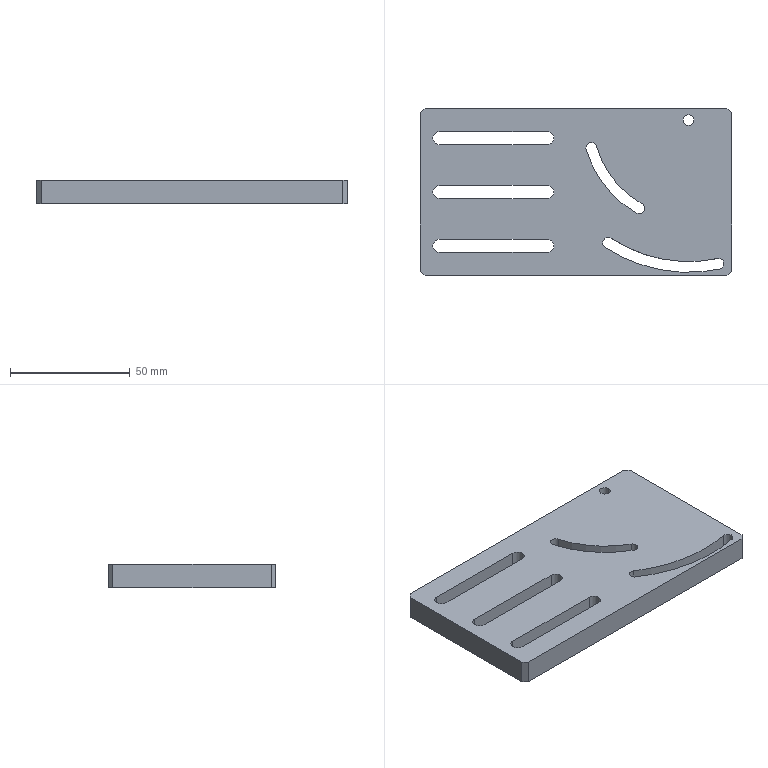Part | NX | 1 solid | 31 faces | box 130 x 70 x 10 mm | volume 78647 mm3 | plane 16 | cylinder 15 | commonest cylinder face diameters 5.5 x6 4.5 x5 79.924 x1 88.924 x1 118.077 x1 127.077 x1
STEP:
#1=CARTESIAN_POINT('',(-63.,35.,10.));
#2=VERTEX_POINT('',#1);
#3=CARTESIAN_POINT('',(-65.,33.,10.));
#4=VERTEX_POINT('',#3);
#5=CARTESIAN_POINT('',(-65.,33.,10.));
#6=DIRECTION('',(-0.7071,-0.7071,0.));
#7=VECTOR('',#6,1000.);
#8=LINE('',#5,#7);
#9=EDGE_CURVE('',#2,#4,#8,.T.);
#10=ORIENTED_EDGE('',*,*,#9,.F.);
#11=CARTESIAN_POINT('',(-63.,35.,0.));
#12=VERTEX_POINT('',#11);
#13=CARTESIAN_POINT('',(-63.,35.,10.));
#14=DIRECTION('',(0.,0.,1.));
#15=VECTOR('',#14,1000.);
#16=LINE('',#13,#15);
#17=EDGE_CURVE('',#12,#2,#16,.T.);
#18=ORIENTED_EDGE('',*,*,#17,.F.);
#19=CARTESIAN_POINT('',(-65.,33.,0.));
#20=VERTEX_POINT('',#19);
#21=CARTESIAN_POINT('',(-49.,49.,0.));
#22=DIRECTION('',(0.7071,0.7071,0.));
#23=VECTOR('',#22,1000.);
#24=LINE('',#21,#23);
#25=EDGE_CURVE('',#20,#12,#24,.T.);
#26=ORIENTED_EDGE('',*,*,#25,.F.);
#27=CARTESIAN_POINT('',(-65.,33.,10.));
#28=DIRECTION('',(0.,0.,-1.));
#29=VECTOR('',#28,1000.);
#30=LINE('',#27,#29);
#31=EDGE_CURVE('',#4,#20,#30,.T.);
#32=ORIENTED_EDGE('',*,*,#31,.F.);
#33=EDGE_LOOP('',(#10,#18,#26,#32));
#34=FACE_BOUND('',#33,.T.);
#35=CARTESIAN_POINT('',(-65.,33.,10.));
#36=DIRECTION('',(0.7071,-0.7071,0.));
#37=DIRECTION('',(0.,0.,-1.));
#38=AXIS2_PLACEMENT_3D('',#35,#36,#37);
#39=PLANE('',#38);
#40=ADVANCED_FACE('',(#34),#39,.F.);
#41=CARTESIAN_POINT('',(-65.,-33.,10.));
#42=VERTEX_POINT('',#41);
#43=CARTESIAN_POINT('',(-63.,-35.,10.));
#44=VERTEX_POINT('',#43);
#45=CARTESIAN_POINT('',(-63.,-35.,10.));
#46=DIRECTION('',(0.7071,-0.7071,0.));
#47=VECTOR('',#46,1000.);
#48=LINE('',#45,#47);
#49=EDGE_CURVE('',#42,#44,#48,.T.);
#50=ORIENTED_EDGE('',*,*,#49,.F.);
#51=CARTESIAN_POINT('',(-65.,-33.,0.));
#52=VERTEX_POINT('',#51);
#53=CARTESIAN_POINT('',(-65.,-33.,10.));
#54=DIRECTION('',(0.,0.,1.));
#55=VECTOR('',#54,1000.);
#56=LINE('',#53,#55);
#57=EDGE_CURVE('',#52,#42,#56,.T.);
#58=ORIENTED_EDGE('',*,*,#57,.F.);
#59=CARTESIAN_POINT('',(-63.,-35.,0.));
#60=VERTEX_POINT('',#59);
#61=CARTESIAN_POINT('',(-49.,-49.,0.));
#62=DIRECTION('',(-0.7071,0.7071,0.));
#63=VECTOR('',#62,1000.);
#64=LINE('',#61,#63);
#65=EDGE_CURVE('',#60,#52,#64,.T.);
#66=ORIENTED_EDGE('',*,*,#65,.F.);
#67=CARTESIAN_POINT('',(-63.,-35.,10.));
#68=DIRECTION('',(0.,0.,-1.));
#69=VECTOR('',#68,1000.);
#70=LINE('',#67,#69);
#71=EDGE_CURVE('',#44,#60,#70,.T.);
#72=ORIENTED_EDGE('',*,*,#71,.F.);
#73=EDGE_LOOP('',(#50,#58,#66,#72));
#74=FACE_BOUND('',#73,.T.);
#75=CARTESIAN_POINT('',(-63.,-35.,10.));
#76=DIRECTION('',(0.7071,0.7071,0.));
#77=DIRECTION('',(0.,0.,-1.));
#78=AXIS2_PLACEMENT_3D('',#75,#76,#77);
#79=PLANE('',#78);
#80=ADVANCED_FACE('',(#74),#79,.F.);
#81=CARTESIAN_POINT('',(65.,33.,10.));
#82=VERTEX_POINT('',#81);
#83=CARTESIAN_POINT('',(63.,35.,10.));
#84=VERTEX_POINT('',#83);
#85=CARTESIAN_POINT('',(63.,35.,10.));
#86=DIRECTION('',(-0.7071,0.7071,0.));
#87=VECTOR('',#86,1000.);
#88=LINE('',#85,#87);
#89=EDGE_CURVE('',#82,#84,#88,.T.);
#90=ORIENTED_EDGE('',*,*,#89,.F.);
#91=CARTESIAN_POINT('',(65.,33.,0.));
#92=VERTEX_POINT('',#91);
#93=CARTESIAN_POINT('',(65.,33.,10.));
#94=DIRECTION('',(0.,0.,1.));
#95=VECTOR('',#94,1000.);
#96=LINE('',#93,#95);
#97=EDGE_CURVE('',#92,#82,#96,.T.);
#98=ORIENTED_EDGE('',*,*,#97,.F.);
#99=CARTESIAN_POINT('',(63.,35.,0.));
#100=VERTEX_POINT('',#99);
#101=CARTESIAN_POINT('',(49.,49.,0.));
#102=DIRECTION('',(0.7071,-0.7071,0.));
#103=VECTOR('',#102,1000.);
#104=LINE('',#101,#103);
#105=EDGE_CURVE('',#100,#92,#104,.T.);
#106=ORIENTED_EDGE('',*,*,#105,.F.);
#107=CARTESIAN_POINT('',(63.,35.,10.));
#108=DIRECTION('',(0.,0.,-1.));
#109=VECTOR('',#108,1000.);
#110=LINE('',#107,#109);
#111=EDGE_CURVE('',#84,#100,#110,.T.);
#112=ORIENTED_EDGE('',*,*,#111,.F.);
#113=EDGE_LOOP('',(#90,#98,#106,#112));
#114=FACE_BOUND('',#113,.T.);
#115=CARTESIAN_POINT('',(63.,35.,10.));
#116=DIRECTION('',(-0.7071,-0.7071,0.));
#117=DIRECTION('',(0.,0.,-1.));
#118=AXIS2_PLACEMENT_3D('',#115,#116,#117);
#119=PLANE('',#118);
#120=ADVANCED_FACE('',(#114),#119,.F.);
#121=CARTESIAN_POINT('',(63.,-35.,10.));
#122=VERTEX_POINT('',#121);
#123=CARTESIAN_POINT('',(65.,-33.,10.));
#124=VERTEX_POINT('',#123);
#125=CARTESIAN_POINT('',(65.,-33.,10.));
#126=DIRECTION('',(0.7071,0.7071,0.));
#127=VECTOR('',#126,1000.);
#128=LINE('',#125,#127);
#129=EDGE_CURVE('',#122,#124,#128,.T.);
#130=ORIENTED_EDGE('',*,*,#129,.F.);
#131=CARTESIAN_POINT('',(63.,-35.,0.));
#132=VERTEX_POINT('',#131);
#133=CARTESIAN_POINT('',(63.,-35.,10.));
#134=DIRECTION('',(0.,0.,1.));
#135=VECTOR('',#134,1000.);
#136=LINE('',#133,#135);
#137=EDGE_CURVE('',#132,#122,#136,.T.);
#138=ORIENTED_EDGE('',*,*,#137,.F.);
#139=CARTESIAN_POINT('',(65.,-33.,0.));
#140=VERTEX_POINT('',#139);
#141=CARTESIAN_POINT('',(49.,-49.,0.));
#142=DIRECTION('',(-0.7071,-0.7071,0.));
#143=VECTOR('',#142,1000.);
#144=LINE('',#141,#143);
#145=EDGE_CURVE('',#140,#132,#144,.T.);
#146=ORIENTED_EDGE('',*,*,#145,.F.);
#147=CARTESIAN_POINT('',(65.,-33.,10.));
#148=DIRECTION('',(0.,0.,-1.));
#149=VECTOR('',#148,1000.);
#150=LINE('',#147,#149);
#151=EDGE_CURVE('',#124,#140,#150,.T.);
#152=ORIENTED_EDGE('',*,*,#151,.F.);
#153=EDGE_LOOP('',(#130,#138,#146,#152));
#154=FACE_BOUND('',#153,.T.);
#155=CARTESIAN_POINT('',(65.,-33.,10.));
#156=DIRECTION('',(-0.7071,0.7071,0.));
#157=DIRECTION('',(0.,0.,-1.));
#158=AXIS2_PLACEMENT_3D('',#155,#156,#157);
#159=PLANE('',#158);
#160=ADVANCED_FACE('',(#154),#159,.F.);
#161=CARTESIAN_POINT('',(-12.,19.75,0.));
#162=VERTEX_POINT('',#161);
#163=CARTESIAN_POINT('',(-57.,19.75,0.));
#164=VERTEX_POINT('',#163);
#165=CARTESIAN_POINT('',(0.,19.75,0.));
#166=DIRECTION('',(-1.,0.,0.));
#167=VECTOR('',#166,1000.);
#168=LINE('',#165,#167);
#169=EDGE_CURVE('',#162,#164,#168,.T.);
#170=ORIENTED_EDGE('',*,*,#169,.T.);
#171=CARTESIAN_POINT('',(-57.,19.75,10.));
#172=VERTEX_POINT('',#171);
#173=CARTESIAN_POINT('',(-57.,19.75,-20.));
#174=DIRECTION('',(0.,0.,1.));
#175=VECTOR('',#174,1000.);
#176=LINE('',#173,#175);
#177=EDGE_CURVE('',#164,#172,#176,.T.);
#178=ORIENTED_EDGE('',*,*,#177,.T.);
#179=CARTESIAN_POINT('',(-12.,19.75,10.));
#180=VERTEX_POINT('',#179);
#181=CARTESIAN_POINT('',(-57.,19.75,10.));
#182=DIRECTION('',(1.,0.,0.));
#183=VECTOR('',#182,1000.);
#184=LINE('',#181,#183);
#185=EDGE_CURVE('',#172,#180,#184,.T.);
#186=ORIENTED_EDGE('',*,*,#185,.T.);
#187=CARTESIAN_POINT('',(-12.,19.75,-20.));
#188=DIRECTION('',(0.,0.,1.));
#189=VECTOR('',#188,1000.);
#190=LINE('',#187,#189);
#191=EDGE_CURVE('',#162,#180,#190,.T.);
#192=ORIENTED_EDGE('',*,*,#191,.F.);
#193=EDGE_LOOP('',(#170,#178,#186,#192));
#194=FACE_BOUND('',#193,.T.);
#195=CARTESIAN_POINT('',(-57.,19.75,-20.));
#196=DIRECTION('',(0.,-1.,0.));
#197=DIRECTION('',(0.,0.,-1.));
#198=AXIS2_PLACEMENT_3D('',#195,#196,#197);
#199=PLANE('',#198);
#200=ADVANCED_FACE('',(#194),#199,.F.);
#201=CARTESIAN_POINT('',(-57.,25.25,0.));
#202=VERTEX_POINT('',#201);
#203=CARTESIAN_POINT('',(-12.,25.25,0.));
#204=VERTEX_POINT('',#203);
#205=CARTESIAN_POINT('',(0.,25.25,0.));
#206=DIRECTION('',(1.,0.,0.));
#207=VECTOR('',#206,1000.);
#208=LINE('',#205,#207);
#209=EDGE_CURVE('',#202,#204,#208,.T.);
#210=ORIENTED_EDGE('',*,*,#209,.T.);
#211=CARTESIAN_POINT('',(-12.,25.25,10.));
#212=VERTEX_POINT('',#211);
#213=CARTESIAN_POINT('',(-12.,25.25,-20.));
#214=DIRECTION('',(0.,0.,1.));
#215=VECTOR('',#214,1000.);
#216=LINE('',#213,#215);
#217=EDGE_CURVE('',#204,#212,#216,.T.);
#218=ORIENTED_EDGE('',*,*,#217,.T.);
#219=CARTESIAN_POINT('',(-57.,25.25,10.));
#220=VERTEX_POINT('',#219);
#221=CARTESIAN_POINT('',(-57.,25.25,10.));
#222=DIRECTION('',(-1.,0.,0.));
#223=VECTOR('',#222,1000.);
#224=LINE('',#221,#223);
#225=EDGE_CURVE('',#212,#220,#224,.T.);
#226=ORIENTED_EDGE('',*,*,#225,.T.);
#227=CARTESIAN_POINT('',(-57.,25.25,-20.));
#228=DIRECTION('',(0.,0.,1.));
#229=VECTOR('',#228,1000.);
#230=LINE('',#227,#229);
#231=EDGE_CURVE('',#202,#220,#230,.T.);
#232=ORIENTED_EDGE('',*,*,#231,.F.);
#233=EDGE_LOOP('',(#210,#218,#226,#232));
#234=FACE_BOUND('',#233,.T.);
#235=CARTESIAN_POINT('',(-57.,25.25,-20.));
#236=DIRECTION('',(0.,1.,0.));
#237=DIRECTION('',(0.,0.,1.));
#238=AXIS2_PLACEMENT_3D('',#235,#236,#237);
#239=PLANE('',#238);
#240=ADVANCED_FACE('',(#234),#239,.F.);
#241=CARTESIAN_POINT('',(-57.,22.5,0.));
#242=DIRECTION('',(0.,0.,-1.));
#243=DIRECTION('',(-1.,0.,0.));
#244=AXIS2_PLACEMENT_3D('',#241,#242,#243);
#245=CIRCLE('',#244,2.75);
#246=EDGE_CURVE('',#164,#202,#245,.T.);
#247=ORIENTED_EDGE('',*,*,#246,.T.);
#248=ORIENTED_EDGE('',*,*,#231,.T.);
#249=CARTESIAN_POINT('',(-57.,22.5,10.));
#250=DIRECTION('',(0.,0.,1.));
#251=DIRECTION('',(1.,0.,0.));
#252=AXIS2_PLACEMENT_3D('',#249,#250,#251);
#253=CIRCLE('',#252,2.75);
#254=EDGE_CURVE('',#220,#172,#253,.T.);
#255=ORIENTED_EDGE('',*,*,#254,.T.);
#256=ORIENTED_EDGE('',*,*,#177,.F.);
#257=EDGE_LOOP('',(#247,#248,#255,#256));
#258=FACE_BOUND('',#257,.T.);
#259=CARTESIAN_POINT('',(-57.,22.5,-20.));
#260=DIRECTION('',(0.,0.,1.));
#261=DIRECTION('',(1.,0.,0.));
#262=AXIS2_PLACEMENT_3D('',#259,#260,#261);
#263=CYLINDRICAL_SURFACE('',#262,2.75);
#264=ADVANCED_FACE('',(#258),#263,.F.);
#265=CARTESIAN_POINT('',(-12.,-25.25,0.));
#266=VERTEX_POINT('',#265);
#267=CARTESIAN_POINT('',(-57.,-25.25,0.));
#268=VERTEX_POINT('',#267);
#269=CARTESIAN_POINT('',(0.,-25.25,0.));
#270=DIRECTION('',(-1.,0.,0.));
#271=VECTOR('',#270,1000.);
#272=LINE('',#269,#271);
#273=EDGE_CURVE('',#266,#268,#272,.T.);
#274=ORIENTED_EDGE('',*,*,#273,.T.);
#275=CARTESIAN_POINT('',(-57.,-25.25,10.));
#276=VERTEX_POINT('',#275);
#277=CARTESIAN_POINT('',(-57.,-25.25,-20.));
#278=DIRECTION('',(0.,0.,1.));
#279=VECTOR('',#278,1000.);
#280=LINE('',#277,#279);
#281=EDGE_CURVE('',#268,#276,#280,.T.);
#282=ORIENTED_EDGE('',*,*,#281,.T.);
#283=CARTESIAN_POINT('',(-12.,-25.25,10.));
#284=VERTEX_POINT('',#283);
#285=CARTESIAN_POINT('',(-57.,-25.25,10.));
#286=DIRECTION('',(1.,0.,0.));
#287=VECTOR('',#286,1000.);
#288=LINE('',#285,#287);
#289=EDGE_CURVE('',#276,#284,#288,.T.);
#290=ORIENTED_EDGE('',*,*,#289,.T.);
#291=CARTESIAN_POINT('',(-12.,-25.25,-20.));
#292=DIRECTION('',(0.,0.,1.));
#293=VECTOR('',#292,1000.);
#294=LINE('',#291,#293);
#295=EDGE_CURVE('',#266,#284,#294,.T.);
#296=ORIENTED_EDGE('',*,*,#295,.F.);
#297=EDGE_LOOP('',(#274,#282,#290,#296));
#298=FACE_BOUND('',#297,.T.);
#299=CARTESIAN_POINT('',(-57.,-25.25,-20.));
#300=DIRECTION('',(0.,-1.,0.));
#301=DIRECTION('',(0.,0.,-1.));
#302=AXIS2_PLACEMENT_3D('',#299,#300,#301);
#303=PLANE('',#302);
#304=ADVANCED_FACE('',(#298),#303,.F.);
#305=CARTESIAN_POINT('',(-57.,-19.75,0.));
#306=VERTEX_POINT('',#305);
#307=CARTESIAN_POINT('',(-12.,-19.75,0.));
#308=VERTEX_POINT('',#307);
#309=CARTESIAN_POINT('',(0.,-19.75,0.));
#310=DIRECTION('',(1.,0.,0.));
#311=VECTOR('',#310,1000.);
#312=LINE('',#309,#311);
#313=EDGE_CURVE('',#306,#308,#312,.T.);
#314=ORIENTED_EDGE('',*,*,#313,.T.);
#315=CARTESIAN_POINT('',(-12.,-19.75,10.));
#316=VERTEX_POINT('',#315);
#317=CARTESIAN_POINT('',(-12.,-19.75,-20.));
#318=DIRECTION('',(0.,0.,1.));
#319=VECTOR('',#318,1000.);
#320=LINE('',#317,#319);
#321=EDGE_CURVE('',#308,#316,#320,.T.);
#322=ORIENTED_EDGE('',*,*,#321,.T.);
#323=CARTESIAN_POINT('',(-57.,-19.75,10.));
#324=VERTEX_POINT('',#323);
#325=CARTESIAN_POINT('',(-57.,-19.75,10.));
#326=DIRECTION('',(-1.,0.,0.));
#327=VECTOR('',#326,1000.);
#328=LINE('',#325,#327);
#329=EDGE_CURVE('',#316,#324,#328,.T.);
#330=ORIENTED_EDGE('',*,*,#329,.T.);
#331=CARTESIAN_POINT('',(-57.,-19.75,-20.));
#332=DIRECTION('',(0.,0.,1.));
#333=VECTOR('',#332,1000.);
#334=LINE('',#331,#333);
#335=EDGE_CURVE('',#306,#324,#334,.T.);
#336=ORIENTED_EDGE('',*,*,#335,.F.);
#337=EDGE_LOOP('',(#314,#322,#330,#336));
#338=FACE_BOUND('',#337,.T.);
#339=CARTESIAN_POINT('',(-57.,-19.75,-20.));
#340=DIRECTION('',(0.,1.,0.));
#341=DIRECTION('',(0.,0.,1.));
#342=AXIS2_PLACEMENT_3D('',#339,#340,#341);
#343=PLANE('',#342);
#344=ADVANCED_FACE('',(#338),#343,.F.);
#345=CARTESIAN_POINT('',(-57.,-22.5,0.));
#346=DIRECTION('',(0.,0.,-1.));
#347=DIRECTION('',(-1.,0.,0.));
#348=AXIS2_PLACEMENT_3D('',#345,#346,#347);
#349=CIRCLE('',#348,2.75);
#350=EDGE_CURVE('',#268,#306,#349,.T.);
#351=ORIENTED_EDGE('',*,*,#350,.T.);
#352=ORIENTED_EDGE('',*,*,#335,.T.);
#353=CARTESIAN_POINT('',(-57.,-22.5,10.));
#354=DIRECTION('',(0.,0.,1.));
#355=DIRECTION('',(-1.,0.,0.));
#356=AXIS2_PLACEMENT_3D('',#353,#354,#355);
#357=CIRCLE('',#356,2.75);
#358=EDGE_CURVE('',#324,#276,#357,.T.);
#359=ORIENTED_EDGE('',*,*,#358,.T.);
#360=ORIENTED_EDGE('',*,*,#281,.F.);
#361=EDGE_LOOP('',(#351,#352,#359,#360));
#362=FACE_BOUND('',#361,.T.);
#363=CARTESIAN_POINT('',(-57.,-22.5,-20.));
#364=DIRECTION('',(0.,0.,1.));
#365=DIRECTION('',(1.,0.,0.));
#366=AXIS2_PLACEMENT_3D('',#363,#364,#365);
#367=CYLINDRICAL_SURFACE('',#366,2.75);
#368=ADVANCED_FACE('',(#362),#367,.F.);
#369=CARTESIAN_POINT('',(-12.,-2.75,0.));
#370=VERTEX_POINT('',#369);
#371=CARTESIAN_POINT('',(-57.,-2.75,0.));
#372=VERTEX_POINT('',#371);
#373=CARTESIAN_POINT('',(0.,-2.75,0.));
#374=DIRECTION('',(-1.,0.,0.));
#375=VECTOR('',#374,1000.);
#376=LINE('',#373,#375);
#377=EDGE_CURVE('',#370,#372,#376,.T.);
#378=ORIENTED_EDGE('',*,*,#377,.T.);
#379=CARTESIAN_POINT('',(-57.,-2.75,10.));
#380=VERTEX_POINT('',#379);
#381=CARTESIAN_POINT('',(-57.,-2.75,-20.));
#382=DIRECTION('',(0.,0.,1.));
#383=VECTOR('',#382,1000.);
#384=LINE('',#381,#383);
#385=EDGE_CURVE('',#372,#380,#384,.T.);
#386=ORIENTED_EDGE('',*,*,#385,.T.);
#387=CARTESIAN_POINT('',(-12.,-2.75,10.));
#388=VERTEX_POINT('',#387);
#389=CARTESIAN_POINT('',(-57.,-2.75,10.));
#390=DIRECTION('',(1.,0.,0.));
#391=VECTOR('',#390,1000.);
#392=LINE('',#389,#391);
#393=EDGE_CURVE('',#380,#388,#392,.T.);
#394=ORIENTED_EDGE('',*,*,#393,.T.);
#395=CARTESIAN_POINT('',(-12.,-2.75,-20.));
#396=DIRECTION('',(0.,0.,1.));
#397=VECTOR('',#396,1000.);
#398=LINE('',#395,#397);
#399=EDGE_CURVE('',#370,#388,#398,.T.);
#400=ORIENTED_EDGE('',*,*,#399,.F.);
#401=EDGE_LOOP('',(#378,#386,#394,#400));
#402=FACE_BOUND('',#401,.T.);
#403=CARTESIAN_POINT('',(-57.,-2.75,-20.));
#404=DIRECTION('',(0.,-1.,0.));
#405=DIRECTION('',(0.,0.,-1.));
#406=AXIS2_PLACEMENT_3D('',#403,#404,#405);
#407=PLANE('',#406);
#408=ADVANCED_FACE('',(#402),#407,.F.);
#409=CARTESIAN_POINT('',(-57.,2.75,0.));
#410=VERTEX_POINT('',#409);
#411=CARTESIAN_POINT('',(-12.,2.75,0.));
#412=VERTEX_POINT('',#411);
#413=CARTESIAN_POINT('',(0.,2.75,0.));
#414=DIRECTION('',(1.,0.,0.));
#415=VECTOR('',#414,1000.);
#416=LINE('',#413,#415);
#417=EDGE_CURVE('',#410,#412,#416,.T.);
#418=ORIENTED_EDGE('',*,*,#417,.T.);
#419=CARTESIAN_POINT('',(-12.,2.75,10.));
#420=VERTEX_POINT('',#419);
#421=CARTESIAN_POINT('',(-12.,2.75,-20.));
#422=DIRECTION('',(0.,0.,1.));
#423=VECTOR('',#422,1000.);
#424=LINE('',#421,#423);
#425=EDGE_CURVE('',#412,#420,#424,.T.);
#426=ORIENTED_EDGE('',*,*,#425,.T.);
#427=CARTESIAN_POINT('',(-57.,2.75,10.));
#428=VERTEX_POINT('',#427);
#429=CARTESIAN_POINT('',(-57.,2.75,10.));
#430=DIRECTION('',(-1.,0.,0.));
#431=VECTOR('',#430,1000.);
#432=LINE('',#429,#431);
#433=EDGE_CURVE('',#420,#428,#432,.T.);
#434=ORIENTED_EDGE('',*,*,#433,.T.);
#435=CARTESIAN_POINT('',(-57.,2.75,-20.));
#436=DIRECTION('',(0.,0.,1.));
#437=VECTOR('',#436,1000.);
#438=LINE('',#435,#437);
#439=EDGE_CURVE('',#410,#428,#438,.T.);
#440=ORIENTED_EDGE('',*,*,#439,.F.);
#441=EDGE_LOOP('',(#418,#426,#434,#440));
#442=FACE_BOUND('',#441,.T.);
#443=CARTESIAN_POINT('',(-57.,2.75,-20.));
#444=DIRECTION('',(0.,1.,0.));
#445=DIRECTION('',(0.,0.,1.));
#446=AXIS2_PLACEMENT_3D('',#443,#444,#445);
#447=PLANE('',#446);
#448=ADVANCED_FACE('',(#442),#447,.F.);
#449=CARTESIAN_POINT('',(-57.,0.,0.));
#450=DIRECTION('',(0.,0.,-1.));
#451=DIRECTION('',(-1.,0.,0.));
#452=AXIS2_PLACEMENT_3D('',#449,#450,#451);
#453=CIRCLE('',#452,2.75);
#454=EDGE_CURVE('',#372,#410,#453,.T.);
#455=ORIENTED_EDGE('',*,*,#454,.T.);
#456=ORIENTED_EDGE('',*,*,#439,.T.);
#457=CARTESIAN_POINT('',(-57.,0.,10.));
#458=DIRECTION('',(0.,0.,1.));
#459=DIRECTION('',(1.,0.,0.));
#460=AXIS2_PLACEMENT_3D('',#457,#458,#459);
#461=CIRCLE('',#460,2.75);
#462=EDGE_CURVE('',#428,#380,#461,.T.);
#463=ORIENTED_EDGE('',*,*,#462,.T.);
#464=ORIENTED_EDGE('',*,*,#385,.F.);
#465=EDGE_LOOP('',(#455,#456,#463,#464));
#466=FACE_BOUND('',#465,.T.);
#467=CARTESIAN_POINT('',(-57.,0.,-20.));
#468=DIRECTION('',(0.,0.,1.));
#469=DIRECTION('',(1.,0.,0.));
#470=AXIS2_PLACEMENT_3D('',#467,#468,#469);
#471=CYLINDRICAL_SURFACE('',#470,2.75);
#472=ADVANCED_FACE('',(#466),#471,.F.);
#473=CARTESIAN_POINT('',(14.645,-19.383,0.));
#474=VERTEX_POINT('',#473);
#475=CARTESIAN_POINT('',(59.041,-27.797,0.));
#476=VERTEX_POINT('',#475);
#477=CARTESIAN_POINT('',(47.,30.,0.));
#478=DIRECTION('',(0.,0.,1.));
#479=DIRECTION('',(-1.,0.,0.));
#480=AXIS2_PLACEMENT_3D('',#477,#478,#479);
#481=CIRCLE('',#480,59.038);
#482=EDGE_CURVE('',#474,#476,#481,.T.);
#483=ORIENTED_EDGE('',*,*,#482,.T.);
#484=CARTESIAN_POINT('',(59.041,-27.797,10.));
#485=VERTEX_POINT('',#484);
#486=CARTESIAN_POINT('',(59.041,-27.797,5.));
#487=DIRECTION('',(0.,0.,1.));
#488=VECTOR('',#487,1000.);
#489=LINE('',#486,#488);
#490=EDGE_CURVE('',#476,#485,#489,.T.);
#491=ORIENTED_EDGE('',*,*,#490,.T.);
#492=CARTESIAN_POINT('',(14.645,-19.383,10.));
#493=VERTEX_POINT('',#492);
#494=CARTESIAN_POINT('',(47.,30.,10.));
#495=DIRECTION('',(0.,0.,-1.));
#496=DIRECTION('',(1.,0.,0.));
#497=AXIS2_PLACEMENT_3D('',#494,#495,#496);
#498=CIRCLE('',#497,59.038);
#499=EDGE_CURVE('',#485,#493,#498,.T.);
#500=ORIENTED_EDGE('',*,*,#499,.T.);
#501=CARTESIAN_POINT('',(14.645,-19.383,-20.));
#502=DIRECTION('',(0.,0.,1.));
#503=VECTOR('',#502,1000.);
#504=LINE('',#501,#503);
#505=EDGE_CURVE('',#474,#493,#504,.T.);
#506=ORIENTED_EDGE('',*,*,#505,.F.);
#507=EDGE_LOOP('',(#483,#491,#500,#506));
#508=FACE_BOUND('',#507,.T.);
#509=CARTESIAN_POINT('',(47.,30.,-20.));
#510=DIRECTION('',(0.,0.,1.));
#511=DIRECTION('',(1.,0.,0.));
#512=AXIS2_PLACEMENT_3D('',#509,#510,#511);
#513=CYLINDRICAL_SURFACE('',#512,59.038);
#514=ADVANCED_FACE('',(#508),#513,.T.);
#515=CARTESIAN_POINT('',(12.179,-23.147,0.));
#516=VERTEX_POINT('',#515);
#517=CARTESIAN_POINT('',(13.412,-21.265,0.));
#518=DIRECTION('',(0.,0.,-1.));
#519=DIRECTION('',(-1.,0.,0.));
#520=AXIS2_PLACEMENT_3D('',#517,#518,#519);
#521=CIRCLE('',#520,2.25);
#522=EDGE_CURVE('',#516,#474,#521,.T.);
#523=ORIENTED_EDGE('',*,*,#522,.T.);
#524=ORIENTED_EDGE('',*,*,#505,.T.);
#525=CARTESIAN_POINT('',(12.179,-23.147,10.));
#526=VERTEX_POINT('',#525);
#527=CARTESIAN_POINT('',(13.412,-21.265,10.));
#528=DIRECTION('',(0.,0.,1.));
#529=DIRECTION('',(1.,0.,0.));
#530=AXIS2_PLACEMENT_3D('',#527,#528,#529);
#531=CIRCLE('',#530,2.25);
#532=EDGE_CURVE('',#493,#526,#531,.T.);
#533=ORIENTED_EDGE('',*,*,#532,.T.);
#534=CARTESIAN_POINT('',(12.179,-23.147,-20.));
#535=DIRECTION('',(0.,0.,1.));
#536=VECTOR('',#535,1000.);
#537=LINE('',#534,#536);
#538=EDGE_CURVE('',#516,#526,#537,.T.);
#539=ORIENTED_EDGE('',*,*,#538,.F.);
#540=EDGE_LOOP('',(#523,#524,#533,#539));
#541=FACE_BOUND('',#540,.T.);
#542=CARTESIAN_POINT('',(13.412,-21.265,-20.));
#543=DIRECTION('',(0.,0.,1.));
#544=DIRECTION('',(1.,0.,0.));
#545=AXIS2_PLACEMENT_3D('',#542,#543,#544);
#546=CYLINDRICAL_SURFACE('',#545,2.25);
#547=ADVANCED_FACE('',(#541),#546,.F.);
#548=CARTESIAN_POINT('',(59.959,-32.203,0.));
#549=VERTEX_POINT('',#548);
#550=CARTESIAN_POINT('',(47.,30.,0.));
#551=DIRECTION('',(0.,0.,-1.));
#552=DIRECTION('',(-1.,0.,0.));
#553=AXIS2_PLACEMENT_3D('',#550,#551,#552);
#554=CIRCLE('',#553,63.538);
#555=EDGE_CURVE('',#549,#516,#554,.T.);
#556=ORIENTED_EDGE('',*,*,#555,.T.);
#557=ORIENTED_EDGE('',*,*,#538,.T.);
#558=CARTESIAN_POINT('',(59.959,-32.203,10.));
#559=VERTEX_POINT('',#558);
#560=CARTESIAN_POINT('',(47.,30.,10.));
#561=DIRECTION('',(0.,0.,1.));
#562=DIRECTION('',(1.,0.,0.));
#563=AXIS2_PLACEMENT_3D('',#560,#561,#562);
#564=CIRCLE('',#563,63.538);
#565=EDGE_CURVE('',#526,#559,#564,.T.);
#566=ORIENTED_EDGE('',*,*,#565,.T.);
#567=CARTESIAN_POINT('',(59.959,-32.203,-5.));
#568=DIRECTION('',(0.,0.,1.));
#569=VECTOR('',#568,1000.);
#570=LINE('',#567,#569);
#571=EDGE_CURVE('',#549,#559,#570,.T.);
#572=ORIENTED_EDGE('',*,*,#571,.F.);
#573=EDGE_LOOP('',(#556,#557,#566,#572));
#574=FACE_BOUND('',#573,.T.);
#575=CARTESIAN_POINT('',(47.,30.,-20.));
#576=DIRECTION('',(0.,0.,1.));
#577=DIRECTION('',(1.,0.,0.));
#578=AXIS2_PLACEMENT_3D('',#575,#576,#577);
#579=CYLINDRICAL_SURFACE('',#578,63.538);
#580=ADVANCED_FACE('',(#574),#579,.F.);
#581=CARTESIAN_POINT('',(8.575,19.022,0.));
#582=VERTEX_POINT('',#581);
#583=CARTESIAN_POINT('',(27.593,-4.933,0.));
#584=VERTEX_POINT('',#583);
#585=CARTESIAN_POINT('',(47.,30.,0.));
#586=DIRECTION('',(0.,0.,1.));
#587=DIRECTION('',(-1.,0.,0.));
#588=AXIS2_PLACEMENT_3D('',#585,#586,#587);
#589=CIRCLE('',#588,39.962);
#590=EDGE_CURVE('',#582,#584,#589,.T.);
#591=ORIENTED_EDGE('',*,*,#590,.T.);
#592=CARTESIAN_POINT('',(27.593,-4.933,10.));
#593=VERTEX_POINT('',#592);
#594=CARTESIAN_POINT('',(27.593,-4.933,5.));
#595=DIRECTION('',(0.,0.,1.));
#596=VECTOR('',#595,1000.);
#597=LINE('',#594,#596);
#598=EDGE_CURVE('',#584,#593,#597,.T.);
#599=ORIENTED_EDGE('',*,*,#598,.T.);
#600=CARTESIAN_POINT('',(8.575,19.022,10.));
#601=VERTEX_POINT('',#600);
#602=CARTESIAN_POINT('',(47.,30.,10.));
#603=DIRECTION('',(0.,0.,-1.));
#604=DIRECTION('',(1.,0.,0.));
#605=AXIS2_PLACEMENT_3D('',#602,#603,#604);
#606=CIRCLE('',#605,39.962);
#607=EDGE_CURVE('',#593,#601,#606,.T.);
#608=ORIENTED_EDGE('',*,*,#607,.T.);
#609=CARTESIAN_POINT('',(8.575,19.022,-20.));
#610=DIRECTION('',(0.,0.,1.));
#611=VECTOR('',#610,1000.);
#612=LINE('',#609,#611);
#613=EDGE_CURVE('',#582,#601,#612,.T.);
#614=ORIENTED_EDGE('',*,*,#613,.F.);
#615=EDGE_LOOP('',(#591,#599,#608,#614));
#616=FACE_BOUND('',#615,.T.);
#617=CARTESIAN_POINT('',(47.,30.,-20.));
#618=DIRECTION('',(0.,0.,1.));
#619=DIRECTION('',(1.,0.,0.));
#620=AXIS2_PLACEMENT_3D('',#617,#618,#619);
#621=CYLINDRICAL_SURFACE('',#620,39.962);
#622=ADVANCED_FACE('',(#616),#621,.T.);
#623=CARTESIAN_POINT('',(4.249,17.785,0.));
#624=VERTEX_POINT('',#623);
#625=CARTESIAN_POINT('',(6.412,18.403,0.));
#626=DIRECTION('',(0.,0.,-1.));
#627=DIRECTION('',(-1.,0.,0.));
#628=AXIS2_PLACEMENT_3D('',#625,#626,#627);
#629=CIRCLE('',#628,2.25);
#630=EDGE_CURVE('',#624,#582,#629,.T.);
#631=ORIENTED_EDGE('',*,*,#630,.T.);
#632=ORIENTED_EDGE('',*,*,#613,.T.);
#633=CARTESIAN_POINT('',(4.249,17.785,10.));
#634=VERTEX_POINT('',#633);
#635=CARTESIAN_POINT('',(6.412,18.403,10.));
#636=DIRECTION('',(0.,0.,1.));
#637=DIRECTION('',(1.,0.,0.));
#638=AXIS2_PLACEMENT_3D('',#635,#636,#637);
#639=CIRCLE('',#638,2.25);
#640=EDGE_CURVE('',#601,#634,#639,.T.);
#641=ORIENTED_EDGE('',*,*,#640,.T.);
#642=CARTESIAN_POINT('',(4.249,17.785,-20.));
#643=DIRECTION('',(0.,0.,1.));
#644=VECTOR('',#643,1000.);
#645=LINE('',#642,#644);
#646=EDGE_CURVE('',#624,#634,#645,.T.);
#647=ORIENTED_EDGE('',*,*,#646,.F.);
#648=EDGE_LOOP('',(#631,#632,#641,#647));
#649=FACE_BOUND('',#648,.T.);
#650=CARTESIAN_POINT('',(6.412,18.403,-20.));
#651=DIRECTION('',(0.,0.,1.));
#652=DIRECTION('',(1.,0.,0.));
#653=AXIS2_PLACEMENT_3D('',#650,#651,#652);
#654=CYLINDRICAL_SURFACE('',#653,2.25);
#655=ADVANCED_FACE('',(#649),#654,.F.);
#656=CARTESIAN_POINT('',(25.407,-8.867,0.));
#657=VERTEX_POINT('',#656);
#658=CARTESIAN_POINT('',(47.,30.,0.));
#659=DIRECTION('',(0.,0.,-1.));
#660=DIRECTION('',(-1.,0.,0.));
#661=AXIS2_PLACEMENT_3D('',#658,#659,#660);
#662=CIRCLE('',#661,44.462);
#663=EDGE_CURVE('',#657,#624,#662,.T.);
#664=ORIENTED_EDGE('',*,*,#663,.T.);
#665=ORIENTED_EDGE('',*,*,#646,.T.);
#666=CARTESIAN_POINT('',(25.407,-8.867,10.));
#667=VERTEX_POINT('',#666);
#668=CARTESIAN_POINT('',(47.,30.,10.));
#669=DIRECTION('',(0.,0.,1.));
#670=DIRECTION('',(1.,0.,0.));
#671=AXIS2_PLACEMENT_3D('',#668,#669,#670);
#672=CIRCLE('',#671,44.462);
#673=EDGE_CURVE('',#634,#667,#672,.T.);
#674=ORIENTED_EDGE('',*,*,#673,.T.);
#675=CARTESIAN_POINT('',(25.407,-8.867,-5.));
#676=DIRECTION('',(0.,0.,1.));
#677=VECTOR('',#676,1000.);
#678=LINE('',#675,#677);
#679=EDGE_CURVE('',#657,#667,#678,.T.);
#680=ORIENTED_EDGE('',*,*,#679,.F.);
#681=EDGE_LOOP('',(#664,#665,#674,#680));
#682=FACE_BOUND('',#681,.T.);
#683=CARTESIAN_POINT('',(47.,30.,-20.));
#684=DIRECTION('',(0.,0.,1.));
#685=DIRECTION('',(1.,0.,0.));
#686=AXIS2_PLACEMENT_3D('',#683,#684,#685);
#687=CYLINDRICAL_SURFACE('',#686,44.462);
#688=ADVANCED_FACE('',(#682),#687,.F.);
#689=CARTESIAN_POINT('',(-65.,-35.,0.));
#690=DIRECTION('',(1.,0.,0.));
#691=VECTOR('',#690,1000.);
#692=LINE('',#689,#691);
#693=EDGE_CURVE('',#60,#132,#692,.T.);
#694=ORIENTED_EDGE('',*,*,#693,.T.);
#695=ORIENTED_EDGE('',*,*,#137,.T.);
#696=CARTESIAN_POINT('',(-65.,-35.,10.));
#697=DIRECTION('',(1.,0.,0.));
#698=VECTOR('',#697,1000.);
#699=LINE('',#696,#698);
#700=EDGE_CURVE('',#44,#122,#699,.T.);
#701=ORIENTED_EDGE('',*,*,#700,.F.);
#702=ORIENTED_EDGE('',*,*,#71,.T.);
#703=EDGE_LOOP('',(#694,#695,#701,#702));
#704=FACE_BOUND('',#703,.T.);
#705=CARTESIAN_POINT('',(-65.,-35.,10.));
#706=DIRECTION('',(0.,1.,0.));
#707=DIRECTION('',(0.,0.,1.));
#708=AXIS2_PLACEMENT_3D('',#705,#706,#707);
#709=PLANE('',#708);
#710=ADVANCED_FACE('',(#704),#709,.F.);
#711=CARTESIAN_POINT('',(-65.,-35.,0.));
#712=DIRECTION('',(0.,-1.,0.));
#713=VECTOR('',#712,1000.);
#714=LINE('',#711,#713);
#715=EDGE_CURVE('',#20,#52,#714,.T.);
#716=ORIENTED_EDGE('',*,*,#715,.T.);
#717=ORIENTED_EDGE('',*,*,#57,.T.);
#718=CARTESIAN_POINT('',(-65.,-35.,10.));
#719=DIRECTION('',(0.,-1.,0.));
#720=VECTOR('',#719,1000.);
#721=LINE('',#718,#720);
#722=EDGE_CURVE('',#4,#42,#721,.T.);
#723=ORIENTED_EDGE('',*,*,#722,.F.);
#724=ORIENTED_EDGE('',*,*,#31,.T.);
#725=EDGE_LOOP('',(#716,#717,#723,#724));
#726=FACE_BOUND('',#725,.T.);
#727=CARTESIAN_POINT('',(-65.,-35.,10.));
#728=DIRECTION('',(1.,0.,0.));
#729=DIRECTION('',(0.,0.,-1.));
#730=AXIS2_PLACEMENT_3D('',#727,#728,#729);
#731=PLANE('',#730);
#732=ADVANCED_FACE('',(#726),#731,.F.);
#733=CARTESIAN_POINT('',(-65.,35.,10.));
#734=DIRECTION('',(-1.,0.,0.));
#735=VECTOR('',#734,1000.);
#736=LINE('',#733,#735);
#737=EDGE_CURVE('',#84,#2,#736,.T.);
#738=ORIENTED_EDGE('',*,*,#737,.F.);
#739=ORIENTED_EDGE('',*,*,#111,.T.);
#740=CARTESIAN_POINT('',(-65.,35.,0.));
#741=DIRECTION('',(-1.,0.,0.));
#742=VECTOR('',#741,1000.);
#743=LINE('',#740,#742);
#744=EDGE_CURVE('',#100,#12,#743,.T.);
#745=ORIENTED_EDGE('',*,*,#744,.T.);
#746=ORIENTED_EDGE('',*,*,#17,.T.);
#747=EDGE_LOOP('',(#738,#739,#745,#746));
#748=FACE_BOUND('',#747,.T.);
#749=CARTESIAN_POINT('',(-65.,35.,10.));
#750=DIRECTION('',(0.,-1.,0.));
#751=DIRECTION('',(0.,0.,-1.));
#752=AXIS2_PLACEMENT_3D('',#749,#750,#751);
#753=PLANE('',#752);
#754=ADVANCED_FACE('',(#748),#753,.F.);
#755=CARTESIAN_POINT('',(65.,-35.,10.));
#756=DIRECTION('',(0.,1.,0.));
#757=VECTOR('',#756,1000.);
#758=LINE('',#755,#757);
#759=EDGE_CURVE('',#124,#82,#758,.T.);
#760=ORIENTED_EDGE('',*,*,#759,.F.);
#761=ORIENTED_EDGE('',*,*,#151,.T.);
#762=CARTESIAN_POINT('',(65.,-35.,0.));
#763=DIRECTION('',(0.,1.,0.));
#764=VECTOR('',#763,1000.);
#765=LINE('',#762,#764);
#766=EDGE_CURVE('',#140,#92,#765,.T.);
#767=ORIENTED_EDGE('',*,*,#766,.T.);
#768=ORIENTED_EDGE('',*,*,#97,.T.);
#769=EDGE_LOOP('',(#760,#761,#767,#768));
#770=FACE_BOUND('',#769,.T.);
#771=CARTESIAN_POINT('',(65.,-35.,10.));
#772=DIRECTION('',(-1.,0.,0.));
#773=DIRECTION('',(0.,0.,1.));
#774=AXIS2_PLACEMENT_3D('',#771,#772,#773);
#775=PLANE('',#774);
#776=ADVANCED_FACE('',(#770),#775,.F.);
#777=ORIENTED_EDGE('',*,*,#555,.F.);
#778=CARTESIAN_POINT('',(59.5,-30.,0.));
#779=DIRECTION('',(0.,0.,-1.));
#780=DIRECTION('',(-1.,0.,0.));
#781=AXIS2_PLACEMENT_3D('',#778,#779,#780);
#782=CIRCLE('',#781,2.25);
#783=EDGE_CURVE('',#476,#549,#782,.T.);
#784=ORIENTED_EDGE('',*,*,#783,.F.);
#785=ORIENTED_EDGE('',*,*,#482,.F.);
#786=ORIENTED_EDGE('',*,*,#522,.F.);
#787=EDGE_LOOP('',(#777,#784,#785,#786));
#788=FACE_BOUND('',#787,.T.);
#789=ORIENTED_EDGE('',*,*,#766,.F.);
#790=ORIENTED_EDGE('',*,*,#145,.T.);
#791=ORIENTED_EDGE('',*,*,#693,.F.);
#792=ORIENTED_EDGE('',*,*,#65,.T.);
#793=ORIENTED_EDGE('',*,*,#715,.F.);
#794=ORIENTED_EDGE('',*,*,#25,.T.);
#795=ORIENTED_EDGE('',*,*,#744,.F.);
#796=ORIENTED_EDGE('',*,*,#105,.T.);
#797=EDGE_LOOP('',(#789,#790,#791,#792,#793,#794,#795,#796));
#798=FACE_BOUND('',#797,.T.);
#799=CARTESIAN_POINT('',(44.75,30.,0.));
#800=VERTEX_POINT('',#799);
#801=CARTESIAN_POINT('',(47.,30.,0.));
#802=DIRECTION('',(0.,0.,-1.));
#803=DIRECTION('',(-1.,0.,0.));
#804=AXIS2_PLACEMENT_3D('',#801,#802,#803);
#805=CIRCLE('',#804,2.25);
#806=EDGE_CURVE('',#800,#800,#805,.T.);
#807=ORIENTED_EDGE('',*,*,#806,.F.);
#808=EDGE_LOOP('',(#807));
#809=FACE_BOUND('',#808,.T.);
#810=ORIENTED_EDGE('',*,*,#663,.F.);
#811=CARTESIAN_POINT('',(26.5,-6.9,0.));
#812=DIRECTION('',(0.,0.,-1.));
#813=DIRECTION('',(-1.,0.,0.));
#814=AXIS2_PLACEMENT_3D('',#811,#812,#813);
#815=CIRCLE('',#814,2.25);
#816=EDGE_CURVE('',#584,#657,#815,.T.);
#817=ORIENTED_EDGE('',*,*,#816,.F.);
#818=ORIENTED_EDGE('',*,*,#590,.F.);
#819=ORIENTED_EDGE('',*,*,#630,.F.);
#820=EDGE_LOOP('',(#810,#817,#818,#819));
#821=FACE_BOUND('',#820,.T.);
#822=ORIENTED_EDGE('',*,*,#454,.F.);
#823=ORIENTED_EDGE('',*,*,#377,.F.);
#824=CARTESIAN_POINT('',(-12.,0.,0.));
#825=DIRECTION('',(0.,0.,-1.));
#826=DIRECTION('',(-1.,0.,0.));
#827=AXIS2_PLACEMENT_3D('',#824,#825,#826);
#828=CIRCLE('',#827,2.75);
#829=EDGE_CURVE('',#412,#370,#828,.T.);
#830=ORIENTED_EDGE('',*,*,#829,.F.);
#831=ORIENTED_EDGE('',*,*,#417,.F.);
#832=EDGE_LOOP('',(#822,#823,#830,#831));
#833=FACE_BOUND('',#832,.T.);
#834=ORIENTED_EDGE('',*,*,#350,.F.);
#835=ORIENTED_EDGE('',*,*,#273,.F.);
#836=CARTESIAN_POINT('',(-12.,-22.5,0.));
#837=DIRECTION('',(0.,0.,-1.));
#838=DIRECTION('',(-1.,0.,0.));
#839=AXIS2_PLACEMENT_3D('',#836,#837,#838);
#840=CIRCLE('',#839,2.75);
#841=EDGE_CURVE('',#308,#266,#840,.T.);
#842=ORIENTED_EDGE('',*,*,#841,.F.);
#843=ORIENTED_EDGE('',*,*,#313,.F.);
#844=EDGE_LOOP('',(#834,#835,#842,#843));
#845=FACE_BOUND('',#844,.T.);
#846=ORIENTED_EDGE('',*,*,#246,.F.);
#847=ORIENTED_EDGE('',*,*,#169,.F.);
#848=CARTESIAN_POINT('',(-12.,22.5,0.));
#849=DIRECTION('',(0.,0.,-1.));
#850=DIRECTION('',(-1.,0.,0.));
#851=AXIS2_PLACEMENT_3D('',#848,#849,#850);
#852=CIRCLE('',#851,2.75);
#853=EDGE_CURVE('',#204,#162,#852,.T.);
#854=ORIENTED_EDGE('',*,*,#853,.F.);
#855=ORIENTED_EDGE('',*,*,#209,.F.);
#856=EDGE_LOOP('',(#846,#847,#854,#855));
#857=FACE_BOUND('',#856,.T.);
#858=CARTESIAN_POINT('',(0.,0.,0.));
#859=DIRECTION('',(0.,0.,-1.));
#860=DIRECTION('',(-1.,0.,0.));
#861=AXIS2_PLACEMENT_3D('',#858,#859,#860);
#862=PLANE('',#861);
#863=ADVANCED_FACE('',(#788,#798,#809,#821,#833,#845,#857),#862,.T.);
#864=CARTESIAN_POINT('',(59.5,-30.,10.));
#865=DIRECTION('',(0.,0.,1.));
#866=DIRECTION('',(1.,0.,0.));
#867=AXIS2_PLACEMENT_3D('',#864,#865,#866);
#868=CIRCLE('',#867,2.25);
#869=EDGE_CURVE('',#559,#485,#868,.T.);
#870=ORIENTED_EDGE('',*,*,#869,.F.);
#871=ORIENTED_EDGE('',*,*,#565,.F.);
#872=ORIENTED_EDGE('',*,*,#532,.F.);
#873=ORIENTED_EDGE('',*,*,#499,.F.);
#874=EDGE_LOOP('',(#870,#871,#872,#873));
#875=FACE_BOUND('',#874,.T.);
#876=CARTESIAN_POINT('',(26.5,-6.9,10.));
#877=DIRECTION('',(0.,0.,1.));
#878=DIRECTION('',(1.,0.,0.));
#879=AXIS2_PLACEMENT_3D('',#876,#877,#878);
#880=CIRCLE('',#879,2.25);
#881=EDGE_CURVE('',#667,#593,#880,.T.);
#882=ORIENTED_EDGE('',*,*,#881,.F.);
#883=ORIENTED_EDGE('',*,*,#673,.F.);
#884=ORIENTED_EDGE('',*,*,#640,.F.);
#885=ORIENTED_EDGE('',*,*,#607,.F.);
#886=EDGE_LOOP('',(#882,#883,#884,#885));
#887=FACE_BOUND('',#886,.T.);
#888=ORIENTED_EDGE('',*,*,#700,.T.);
#889=ORIENTED_EDGE('',*,*,#129,.T.);
#890=ORIENTED_EDGE('',*,*,#759,.T.);
#891=ORIENTED_EDGE('',*,*,#89,.T.);
#892=ORIENTED_EDGE('',*,*,#737,.T.);
#893=ORIENTED_EDGE('',*,*,#9,.T.);
#894=ORIENTED_EDGE('',*,*,#722,.T.);
#895=ORIENTED_EDGE('',*,*,#49,.T.);
#896=EDGE_LOOP('',(#888,#889,#890,#891,#892,#893,#894,#895));
#897=FACE_BOUND('',#896,.T.);
#898=CARTESIAN_POINT('',(49.25,30.,10.));
#899=VERTEX_POINT('',#898);
#900=CARTESIAN_POINT('',(47.,30.,10.));
#901=DIRECTION('',(0.,0.,1.));
#902=DIRECTION('',(1.,0.,0.));
#903=AXIS2_PLACEMENT_3D('',#900,#901,#902);
#904=CIRCLE('',#903,2.25);
#905=EDGE_CURVE('',#899,#899,#904,.T.);
#906=ORIENTED_EDGE('',*,*,#905,.F.);
#907=EDGE_LOOP('',(#906));
#908=FACE_BOUND('',#907,.T.);
#909=ORIENTED_EDGE('',*,*,#393,.F.);
#910=ORIENTED_EDGE('',*,*,#462,.F.);
#911=ORIENTED_EDGE('',*,*,#433,.F.);
#912=CARTESIAN_POINT('',(-12.,0.,10.));
#913=DIRECTION('',(0.,0.,1.));
#914=DIRECTION('',(1.,0.,0.));
#915=AXIS2_PLACEMENT_3D('',#912,#913,#914);
#916=CIRCLE('',#915,2.75);
#917=EDGE_CURVE('',#388,#420,#916,.T.);
#918=ORIENTED_EDGE('',*,*,#917,.F.);
#919=EDGE_LOOP('',(#909,#910,#911,#918));
#920=FACE_BOUND('',#919,.T.);
#921=ORIENTED_EDGE('',*,*,#289,.F.);
#922=ORIENTED_EDGE('',*,*,#358,.F.);
#923=ORIENTED_EDGE('',*,*,#329,.F.);
#924=CARTESIAN_POINT('',(-12.,-22.5,10.));
#925=DIRECTION('',(0.,0.,1.));
#926=DIRECTION('',(-1.,0.,0.));
#927=AXIS2_PLACEMENT_3D('',#924,#925,#926);
#928=CIRCLE('',#927,2.75);
#929=EDGE_CURVE('',#284,#316,#928,.T.);
#930=ORIENTED_EDGE('',*,*,#929,.F.);
#931=EDGE_LOOP('',(#921,#922,#923,#930));
#932=FACE_BOUND('',#931,.T.);
#933=ORIENTED_EDGE('',*,*,#185,.F.);
#934=ORIENTED_EDGE('',*,*,#254,.F.);
#935=ORIENTED_EDGE('',*,*,#225,.F.);
#936=CARTESIAN_POINT('',(-12.,22.5,10.));
#937=DIRECTION('',(0.,0.,1.));
#938=DIRECTION('',(1.,0.,0.));
#939=AXIS2_PLACEMENT_3D('',#936,#937,#938);
#940=CIRCLE('',#939,2.75);
#941=EDGE_CURVE('',#180,#212,#940,.T.);
#942=ORIENTED_EDGE('',*,*,#941,.F.);
#943=EDGE_LOOP('',(#933,#934,#935,#942));
#944=FACE_BOUND('',#943,.T.);
#945=CARTESIAN_POINT('',(0.,0.,10.));
#946=DIRECTION('',(0.,0.,-1.));
#947=DIRECTION('',(-1.,0.,0.));
#948=AXIS2_PLACEMENT_3D('',#945,#946,#947);
#949=PLANE('',#948);
#950=ADVANCED_FACE('',(#875,#887,#897,#908,#920,#932,#944),#949,.F.);
#951=ORIENTED_EDGE('',*,*,#783,.T.);
#952=ORIENTED_EDGE('',*,*,#571,.T.);
#953=ORIENTED_EDGE('',*,*,#869,.T.);
#954=ORIENTED_EDGE('',*,*,#490,.F.);
#955=EDGE_LOOP('',(#951,#952,#953,#954));
#956=FACE_BOUND('',#955,.T.);
#957=CARTESIAN_POINT('',(59.5,-30.,-20.));
#958=DIRECTION('',(0.,0.,1.));
#959=DIRECTION('',(1.,0.,0.));
#960=AXIS2_PLACEMENT_3D('',#957,#958,#959);
#961=CYLINDRICAL_SURFACE('',#960,2.25);
#962=ADVANCED_FACE('',(#956),#961,.F.);
#963=ORIENTED_EDGE('',*,*,#816,.T.);
#964=ORIENTED_EDGE('',*,*,#679,.T.);
#965=ORIENTED_EDGE('',*,*,#881,.T.);
#966=ORIENTED_EDGE('',*,*,#598,.F.);
#967=EDGE_LOOP('',(#963,#964,#965,#966));
#968=FACE_BOUND('',#967,.T.);
#969=CARTESIAN_POINT('',(26.5,-6.9,-20.));
#970=DIRECTION('',(0.,0.,1.));
#971=DIRECTION('',(1.,0.,0.));
#972=AXIS2_PLACEMENT_3D('',#969,#970,#971);
#973=CYLINDRICAL_SURFACE('',#972,2.25);
#974=ADVANCED_FACE('',(#968),#973,.F.);
#975=ORIENTED_EDGE('',*,*,#806,.T.);
#976=EDGE_LOOP('',(#975));
#977=FACE_BOUND('',#976,.T.);
#978=ORIENTED_EDGE('',*,*,#905,.T.);
#979=EDGE_LOOP('',(#978));
#980=FACE_BOUND('',#979,.T.);
#981=CARTESIAN_POINT('',(47.,30.,-20.));
#982=DIRECTION('',(0.,0.,1.));
#983=DIRECTION('',(1.,0.,0.));
#984=AXIS2_PLACEMENT_3D('',#981,#982,#983);
#985=CYLINDRICAL_SURFACE('',#984,2.25);
#986=ADVANCED_FACE('',(#977,#980),#985,.F.);
#987=ORIENTED_EDGE('',*,*,#829,.T.);
#988=ORIENTED_EDGE('',*,*,#399,.T.);
#989=ORIENTED_EDGE('',*,*,#917,.T.);
#990=ORIENTED_EDGE('',*,*,#425,.F.);
#991=EDGE_LOOP('',(#987,#988,#989,#990));
#992=FACE_BOUND('',#991,.T.);
#993=CARTESIAN_POINT('',(-12.,0.,-20.));
#994=DIRECTION('',(0.,0.,1.));
#995=DIRECTION('',(1.,0.,0.));
#996=AXIS2_PLACEMENT_3D('',#993,#994,#995);
#997=CYLINDRICAL_SURFACE('',#996,2.75);
#998=ADVANCED_FACE('',(#992),#997,.F.);
#999=ORIENTED_EDGE('',*,*,#841,.T.);
#1000=ORIENTED_EDGE('',*,*,#295,.T.);
#1001=ORIENTED_EDGE('',*,*,#929,.T.);
#1002=ORIENTED_EDGE('',*,*,#321,.F.);
#1003=EDGE_LOOP('',(#999,#1000,#1001,#1002));
#1004=FACE_BOUND('',#1003,.T.);
#1005=CARTESIAN_POINT('',(-12.,-22.5,-20.));
#1006=DIRECTION('',(0.,0.,1.));
#1007=DIRECTION('',(1.,0.,0.));
#1008=AXIS2_PLACEMENT_3D('',#1005,#1006,#1007);
#1009=CYLINDRICAL_SURFACE('',#1008,2.75);
#1010=ADVANCED_FACE('',(#1004),#1009,.F.);
#1011=ORIENTED_EDGE('',*,*,#853,.T.);
#1012=ORIENTED_EDGE('',*,*,#191,.T.);
#1013=ORIENTED_EDGE('',*,*,#941,.T.);
#1014=ORIENTED_EDGE('',*,*,#217,.F.);
#1015=EDGE_LOOP('',(#1011,#1012,#1013,#1014));
#1016=FACE_BOUND('',#1015,.T.);
#1017=CARTESIAN_POINT('',(-12.,22.5,-20.));
#1018=DIRECTION('',(0.,0.,1.));
#1019=DIRECTION('',(1.,0.,0.));
#1020=AXIS2_PLACEMENT_3D('',#1017,#1018,#1019);
#1021=CYLINDRICAL_SURFACE('',#1020,2.75);
#1022=ADVANCED_FACE('',(#1016),#1021,.F.);
#1023=CLOSED_SHELL('',(#40,#80,#120,#160,#200,#240,#264,#304,#344,#368,#408,#448,#472,#514,#547,#580,#622,#655,#688,#710,#732,#754,#776,#863,#950,#962,#974,#986,#998,#1010,#1022));
#1024=MANIFOLD_SOLID_BREP('',#1023);
#1025=(LENGTH_UNIT()NAMED_UNIT(*)SI_UNIT(.MILLI.,.METRE.));
#1026=UNCERTAINTY_MEASURE_WITH_UNIT(LENGTH_MEASURE(0.00001),#1025,'','');
#1027=(NAMED_UNIT(*)PLANE_ANGLE_UNIT()SI_UNIT($,.RADIAN.));
#1028=(NAMED_UNIT(*)SI_UNIT($,.STERADIAN.)SOLID_ANGLE_UNIT());
#1029=(GEOMETRIC_REPRESENTATION_CONTEXT(3)GLOBAL_UNCERTAINTY_ASSIGNED_CONTEXT((#1026))GLOBAL_UNIT_ASSIGNED_CONTEXT((#1025,#1027,#1028))REPRESENTATION_CONTEXT('',''));
#1030=ADVANCED_BREP_SHAPE_REPRESENTATION('',(#1024),#1029);